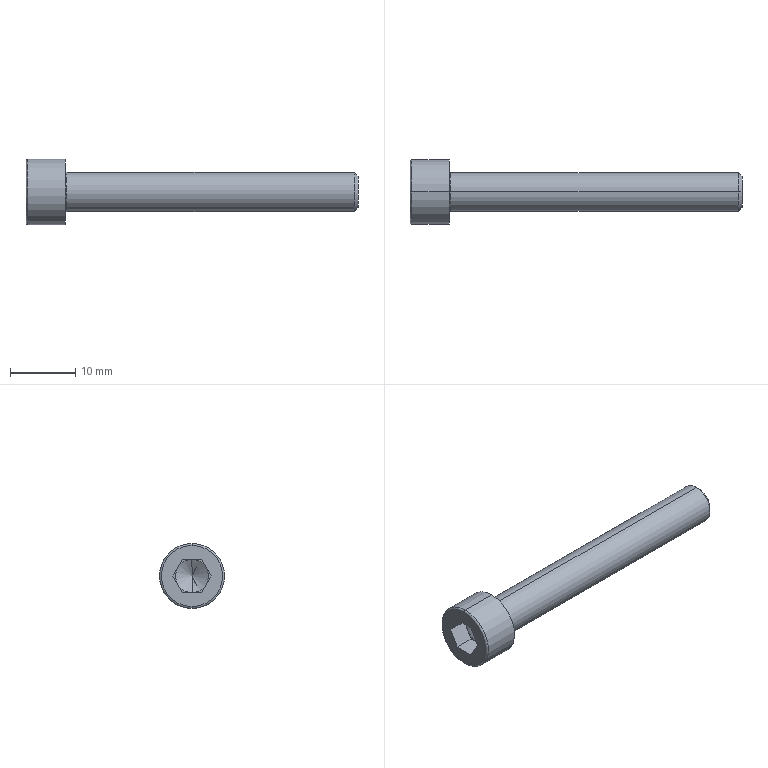Part | STEP file | socket head cap screw_iso_ISO 4762 M6 x 45 --- 24N | 1 solid | 27 faces | box 51 x 10 x 10 mm | volume 1663 mm3 | plane 15 | cone 4 | torus 4 | cylinder 4 | commonest cylinder face diameters 6 x2 10 x2